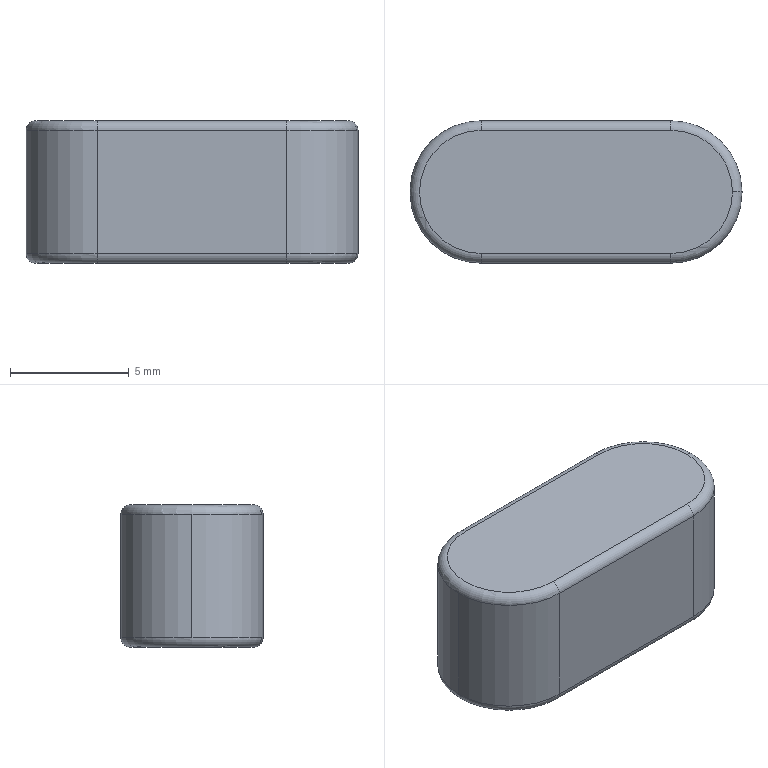Part | SolidWorks | features Extrusion 1, Fillet 1 | 1 solid | 17 faces | box 14 x 6 x 6 mm | volume 455.291 mm3 | cylinder 7 | torus 6 | plane 4 | commonest cylinder face diameters 0.8 x4 6 x3
STEP:
#1=CARTESIAN_POINT('',(6.6,0.,0.));
#2=VERTEX_POINT('',#1);
#3=CARTESIAN_POINT('',(4.,-2.6,0.));
#4=VERTEX_POINT('',#3);
#5=CARTESIAN_POINT('',(4.,0.,0.));
#6=DIRECTION('',(0.,0.,-1.));
#7=DIRECTION('',(1.,0.,0.));
#8=AXIS2_PLACEMENT_3D('',#5,#6,#7);
#9=CIRCLE('',#8,2.6);
#10=EDGE_CURVE('',#2,#4,#9,.T.);
#11=ORIENTED_EDGE('',*,*,#10,.F.);
#12=CARTESIAN_POINT('',(7.,0.,0.4));
#13=VERTEX_POINT('',#12);
#14=CARTESIAN_POINT('',(6.6,0.,0.4));
#15=DIRECTION('',(0.,-1.,0.));
#16=DIRECTION('',(0.,0.,-1.));
#17=AXIS2_PLACEMENT_3D('',#14,#15,#16);
#18=CIRCLE('',#17,0.4);
#19=EDGE_CURVE('',#2,#13,#18,.T.);
#20=ORIENTED_EDGE('',*,*,#19,.T.);
#21=CARTESIAN_POINT('',(4.,-3.,0.4));
#22=VERTEX_POINT('',#21);
#23=CARTESIAN_POINT('',(4.,0.,0.4));
#24=DIRECTION('',(0.,0.,1.));
#25=DIRECTION('',(1.,0.,0.));
#26=AXIS2_PLACEMENT_3D('',#23,#24,#25);
#27=CIRCLE('',#26,3.);
#28=EDGE_CURVE('',#22,#13,#27,.T.);
#29=ORIENTED_EDGE('',*,*,#28,.F.);
#30=CARTESIAN_POINT('',(4.,-2.6,0.4));
#31=DIRECTION('',(1.,0.,0.));
#32=DIRECTION('',(0.,0.,-1.));
#33=AXIS2_PLACEMENT_3D('',#30,#31,#32);
#34=CIRCLE('',#33,0.4);
#35=EDGE_CURVE('',#22,#4,#34,.T.);
#36=ORIENTED_EDGE('',*,*,#35,.T.);
#37=EDGE_LOOP('',(#11,#20,#29,#36));
#38=FACE_OUTER_BOUND('',#37,.T.);
#39=CARTESIAN_POINT('',(4.,0.,0.4));
#40=DIRECTION('',(0.,0.,1.));
#41=DIRECTION('',(1.,0.,0.));
#42=AXIS2_PLACEMENT_3D('',#39,#40,#41);
#43=TOROIDAL_SURFACE('',#42,2.6,0.4);
#44=ADVANCED_FACE('',(#38),#43,.T.);
#45=CARTESIAN_POINT('',(7.,0.,5.6));
#46=VERTEX_POINT('',#45);
#47=CARTESIAN_POINT('',(4.,-3.,5.6));
#48=VERTEX_POINT('',#47);
#49=CARTESIAN_POINT('',(4.,0.,5.6));
#50=DIRECTION('',(0.,0.,-1.));
#51=DIRECTION('',(1.,0.,0.));
#52=AXIS2_PLACEMENT_3D('',#49,#50,#51);
#53=CIRCLE('',#52,3.);
#54=EDGE_CURVE('',#46,#48,#53,.T.);
#55=ORIENTED_EDGE('',*,*,#54,.F.);
#56=CARTESIAN_POINT('',(6.6,0.,6.));
#57=VERTEX_POINT('',#56);
#58=CARTESIAN_POINT('',(6.6,0.,5.6));
#59=DIRECTION('',(0.,-1.,0.));
#60=DIRECTION('',(0.,0.,-1.));
#61=AXIS2_PLACEMENT_3D('',#58,#59,#60);
#62=CIRCLE('',#61,0.4);
#63=EDGE_CURVE('',#46,#57,#62,.T.);
#64=ORIENTED_EDGE('',*,*,#63,.T.);
#65=CARTESIAN_POINT('',(4.,-2.6,6.));
#66=VERTEX_POINT('',#65);
#67=CARTESIAN_POINT('',(4.,0.,6.));
#68=DIRECTION('',(0.,0.,1.));
#69=DIRECTION('',(1.,0.,0.));
#70=AXIS2_PLACEMENT_3D('',#67,#68,#69);
#71=CIRCLE('',#70,2.6);
#72=EDGE_CURVE('',#66,#57,#71,.T.);
#73=ORIENTED_EDGE('',*,*,#72,.F.);
#74=CARTESIAN_POINT('',(4.,-2.6,5.6));
#75=DIRECTION('',(1.,0.,0.));
#76=DIRECTION('',(0.,0.,-1.));
#77=AXIS2_PLACEMENT_3D('',#74,#75,#76);
#78=CIRCLE('',#77,0.4);
#79=EDGE_CURVE('',#66,#48,#78,.T.);
#80=ORIENTED_EDGE('',*,*,#79,.T.);
#81=EDGE_LOOP('',(#55,#64,#73,#80));
#82=FACE_OUTER_BOUND('',#81,.T.);
#83=CARTESIAN_POINT('',(4.,0.,5.6));
#84=DIRECTION('',(0.,0.,1.));
#85=DIRECTION('',(1.,0.,0.));
#86=AXIS2_PLACEMENT_3D('',#83,#84,#85);
#87=TOROIDAL_SURFACE('',#86,2.6,0.4);
#88=ADVANCED_FACE('',(#82),#87,.T.);
#89=CARTESIAN_POINT('',(-4.,-3.,5.6));
#90=VERTEX_POINT('',#89);
#91=CARTESIAN_POINT('',(-7.,0.,5.6));
#92=VERTEX_POINT('',#91);
#93=CARTESIAN_POINT('',(-4.,0.,5.6));
#94=DIRECTION('',(0.,0.,-1.));
#95=DIRECTION('',(1.,0.,0.));
#96=AXIS2_PLACEMENT_3D('',#93,#94,#95);
#97=CIRCLE('',#96,3.);
#98=EDGE_CURVE('',#90,#92,#97,.T.);
#99=ORIENTED_EDGE('',*,*,#98,.T.);
#100=CARTESIAN_POINT('',(-7.,0.,0.4));
#101=VERTEX_POINT('',#100);
#102=CARTESIAN_POINT('',(-7.,0.,6.));
#103=DIRECTION('',(0.,0.,-1.));
#104=VECTOR('',#103,1000.);
#105=LINE('',#102,#104);
#106=EDGE_CURVE('',#92,#101,#105,.T.);
#107=ORIENTED_EDGE('',*,*,#106,.T.);
#108=CARTESIAN_POINT('',(-4.,-3.,0.4));
#109=VERTEX_POINT('',#108);
#110=CARTESIAN_POINT('',(-4.,0.,0.4));
#111=DIRECTION('',(0.,0.,1.));
#112=DIRECTION('',(1.,0.,0.));
#113=AXIS2_PLACEMENT_3D('',#110,#111,#112);
#114=CIRCLE('',#113,3.);
#115=EDGE_CURVE('',#101,#109,#114,.T.);
#116=ORIENTED_EDGE('',*,*,#115,.T.);
#117=CARTESIAN_POINT('',(-4.,-3.,6.));
#118=DIRECTION('',(0.,0.,-1.));
#119=VECTOR('',#118,1000.);
#120=LINE('',#117,#119);
#121=EDGE_CURVE('',#90,#109,#120,.T.);
#122=ORIENTED_EDGE('',*,*,#121,.F.);
#123=EDGE_LOOP('',(#99,#107,#116,#122));
#124=FACE_OUTER_BOUND('',#123,.T.);
#125=CARTESIAN_POINT('',(-4.,0.,6.));
#126=DIRECTION('',(0.,0.,-1.));
#127=DIRECTION('',(-1.,0.,0.));
#128=AXIS2_PLACEMENT_3D('',#125,#126,#127);
#129=CYLINDRICAL_SURFACE('',#128,3.);
#130=ADVANCED_FACE('',(#124),#129,.T.);
#131=ORIENTED_EDGE('',*,*,#106,.F.);
#132=CARTESIAN_POINT('',(-4.,3.,5.6));
#133=VERTEX_POINT('',#132);
#134=CARTESIAN_POINT('',(-4.,0.,5.6));
#135=DIRECTION('',(0.,0.,-1.));
#136=DIRECTION('',(1.,0.,0.));
#137=AXIS2_PLACEMENT_3D('',#134,#135,#136);
#138=CIRCLE('',#137,3.);
#139=EDGE_CURVE('',#92,#133,#138,.T.);
#140=ORIENTED_EDGE('',*,*,#139,.T.);
#141=CARTESIAN_POINT('',(-4.,3.,0.4));
#142=VERTEX_POINT('',#141);
#143=CARTESIAN_POINT('',(-4.,3.,6.));
#144=DIRECTION('',(0.,0.,-1.));
#145=VECTOR('',#144,1000.);
#146=LINE('',#143,#145);
#147=EDGE_CURVE('',#133,#142,#146,.T.);
#148=ORIENTED_EDGE('',*,*,#147,.T.);
#149=CARTESIAN_POINT('',(-4.,0.,0.4));
#150=DIRECTION('',(0.,0.,1.));
#151=DIRECTION('',(1.,0.,0.));
#152=AXIS2_PLACEMENT_3D('',#149,#150,#151);
#153=CIRCLE('',#152,3.);
#154=EDGE_CURVE('',#142,#101,#153,.T.);
#155=ORIENTED_EDGE('',*,*,#154,.T.);
#156=EDGE_LOOP('',(#131,#140,#148,#155));
#157=FACE_OUTER_BOUND('',#156,.T.);
#158=CARTESIAN_POINT('',(-4.,0.,6.));
#159=DIRECTION('',(0.,0.,-1.));
#160=DIRECTION('',(-1.,0.,0.));
#161=AXIS2_PLACEMENT_3D('',#158,#159,#160);
#162=CYLINDRICAL_SURFACE('',#161,3.);
#163=ADVANCED_FACE('',(#157),#162,.T.);
#164=CARTESIAN_POINT('',(4.,-3.,6.));
#165=DIRECTION('',(0.,0.,-1.));
#166=VECTOR('',#165,1000.);
#167=LINE('',#164,#166);
#168=EDGE_CURVE('',#48,#22,#167,.T.);
#169=ORIENTED_EDGE('',*,*,#168,.F.);
#170=CARTESIAN_POINT('',(-4.,-3.,5.6));
#171=DIRECTION('',(-1.,0.,0.));
#172=VECTOR('',#171,1000.);
#173=LINE('',#170,#172);
#174=EDGE_CURVE('',#48,#90,#173,.T.);
#175=ORIENTED_EDGE('',*,*,#174,.T.);
#176=ORIENTED_EDGE('',*,*,#121,.T.);
#177=CARTESIAN_POINT('',(-4.,-3.,0.4));
#178=DIRECTION('',(1.,0.,0.));
#179=VECTOR('',#178,1000.);
#180=LINE('',#177,#179);
#181=EDGE_CURVE('',#109,#22,#180,.T.);
#182=ORIENTED_EDGE('',*,*,#181,.T.);
#183=EDGE_LOOP('',(#169,#175,#176,#182));
#184=FACE_OUTER_BOUND('',#183,.T.);
#185=CARTESIAN_POINT('',(-4.,-3.,6.));
#186=DIRECTION('',(0.,1.,0.));
#187=DIRECTION('',(-1.,0.,0.));
#188=AXIS2_PLACEMENT_3D('',#185,#186,#187);
#189=PLANE('',#188);
#190=ADVANCED_FACE('',(#184),#189,.F.);
#191=CARTESIAN_POINT('',(4.,3.,5.6));
#192=VERTEX_POINT('',#191);
#193=CARTESIAN_POINT('',(4.,3.,0.4));
#194=VERTEX_POINT('',#193);
#195=CARTESIAN_POINT('',(4.,3.,6.));
#196=DIRECTION('',(0.,0.,-1.));
#197=VECTOR('',#196,1000.);
#198=LINE('',#195,#197);
#199=EDGE_CURVE('',#192,#194,#198,.T.);
#200=ORIENTED_EDGE('',*,*,#199,.F.);
#201=CARTESIAN_POINT('',(4.,0.,5.6));
#202=DIRECTION('',(0.,0.,-1.));
#203=DIRECTION('',(1.,0.,0.));
#204=AXIS2_PLACEMENT_3D('',#201,#202,#203);
#205=CIRCLE('',#204,3.);
#206=EDGE_CURVE('',#192,#46,#205,.T.);
#207=ORIENTED_EDGE('',*,*,#206,.T.);
#208=ORIENTED_EDGE('',*,*,#54,.T.);
#209=ORIENTED_EDGE('',*,*,#168,.T.);
#210=ORIENTED_EDGE('',*,*,#28,.T.);
#211=CARTESIAN_POINT('',(4.,0.,0.4));
#212=DIRECTION('',(0.,0.,1.));
#213=DIRECTION('',(1.,0.,0.));
#214=AXIS2_PLACEMENT_3D('',#211,#212,#213);
#215=CIRCLE('',#214,3.);
#216=EDGE_CURVE('',#13,#194,#215,.T.);
#217=ORIENTED_EDGE('',*,*,#216,.T.);
#218=EDGE_LOOP('',(#200,#207,#208,#209,#210,#217));
#219=FACE_OUTER_BOUND('',#218,.T.);
#220=CARTESIAN_POINT('',(4.,0.,6.));
#221=DIRECTION('',(0.,0.,-1.));
#222=DIRECTION('',(-1.,0.,0.));
#223=AXIS2_PLACEMENT_3D('',#220,#221,#222);
#224=CYLINDRICAL_SURFACE('',#223,3.);
#225=ADVANCED_FACE('',(#219),#224,.T.);
#226=ORIENTED_EDGE('',*,*,#147,.F.);
#227=CARTESIAN_POINT('',(4.,3.,5.6));
#228=DIRECTION('',(1.,0.,0.));
#229=VECTOR('',#228,1000.);
#230=LINE('',#227,#229);
#231=EDGE_CURVE('',#133,#192,#230,.T.);
#232=ORIENTED_EDGE('',*,*,#231,.T.);
#233=ORIENTED_EDGE('',*,*,#199,.T.);
#234=CARTESIAN_POINT('',(-4.,3.,0.4));
#235=DIRECTION('',(-1.,0.,0.));
#236=VECTOR('',#235,1000.);
#237=LINE('',#234,#236);
#238=EDGE_CURVE('',#194,#142,#237,.T.);
#239=ORIENTED_EDGE('',*,*,#238,.T.);
#240=EDGE_LOOP('',(#226,#232,#233,#239));
#241=FACE_OUTER_BOUND('',#240,.T.);
#242=CARTESIAN_POINT('',(-4.,3.,6.));
#243=DIRECTION('',(0.,-1.,0.));
#244=DIRECTION('',(1.,0.,0.));
#245=AXIS2_PLACEMENT_3D('',#242,#243,#244);
#246=PLANE('',#245);
#247=ADVANCED_FACE('',(#241),#246,.F.);
#248=CARTESIAN_POINT('',(-4.,-2.6,6.));
#249=VERTEX_POINT('',#248);
#250=CARTESIAN_POINT('',(4.,-2.6,6.));
#251=DIRECTION('',(1.,0.,0.));
#252=VECTOR('',#251,1000.);
#253=LINE('',#250,#252);
#254=EDGE_CURVE('',#249,#66,#253,.T.);
#255=ORIENTED_EDGE('',*,*,#254,.T.);
#256=ORIENTED_EDGE('',*,*,#72,.T.);
#257=CARTESIAN_POINT('',(4.,2.6,6.));
#258=VERTEX_POINT('',#257);
#259=CARTESIAN_POINT('',(4.,0.,6.));
#260=DIRECTION('',(0.,0.,1.));
#261=DIRECTION('',(1.,0.,0.));
#262=AXIS2_PLACEMENT_3D('',#259,#260,#261);
#263=CIRCLE('',#262,2.6);
#264=EDGE_CURVE('',#57,#258,#263,.T.);
#265=ORIENTED_EDGE('',*,*,#264,.T.);
#266=CARTESIAN_POINT('',(-4.,2.6,6.));
#267=VERTEX_POINT('',#266);
#268=CARTESIAN_POINT('',(-4.,2.6,6.));
#269=DIRECTION('',(-1.,0.,0.));
#270=VECTOR('',#269,1000.);
#271=LINE('',#268,#270);
#272=EDGE_CURVE('',#258,#267,#271,.T.);
#273=ORIENTED_EDGE('',*,*,#272,.T.);
#274=CARTESIAN_POINT('',(-4.,0.,6.));
#275=DIRECTION('',(0.,0.,1.));
#276=DIRECTION('',(1.,0.,0.));
#277=AXIS2_PLACEMENT_3D('',#274,#275,#276);
#278=CIRCLE('',#277,2.6);
#279=EDGE_CURVE('',#267,#249,#278,.T.);
#280=ORIENTED_EDGE('',*,*,#279,.T.);
#281=EDGE_LOOP('',(#255,#256,#265,#273,#280));
#282=FACE_OUTER_BOUND('',#281,.T.);
#283=CARTESIAN_POINT('',(-4.,0.,6.));
#284=DIRECTION('',(0.,0.,1.));
#285=DIRECTION('',(1.,0.,0.));
#286=AXIS2_PLACEMENT_3D('',#283,#284,#285);
#287=PLANE('',#286);
#288=ADVANCED_FACE('',(#282),#287,.T.);
#289=CARTESIAN_POINT('',(-4.,2.6,0.));
#290=VERTEX_POINT('',#289);
#291=CARTESIAN_POINT('',(4.,2.6,0.));
#292=VERTEX_POINT('',#291);
#293=CARTESIAN_POINT('',(-4.,2.6,0.));
#294=DIRECTION('',(1.,0.,0.));
#295=VECTOR('',#294,1000.);
#296=LINE('',#293,#295);
#297=EDGE_CURVE('',#290,#292,#296,.T.);
#298=ORIENTED_EDGE('',*,*,#297,.T.);
#299=CARTESIAN_POINT('',(4.,0.,0.));
#300=DIRECTION('',(0.,0.,-1.));
#301=DIRECTION('',(1.,0.,0.));
#302=AXIS2_PLACEMENT_3D('',#299,#300,#301);
#303=CIRCLE('',#302,2.6);
#304=EDGE_CURVE('',#292,#2,#303,.T.);
#305=ORIENTED_EDGE('',*,*,#304,.T.);
#306=ORIENTED_EDGE('',*,*,#10,.T.);
#307=CARTESIAN_POINT('',(-4.,-2.6,0.));
#308=VERTEX_POINT('',#307);
#309=CARTESIAN_POINT('',(-4.,-2.6,0.));
#310=DIRECTION('',(-1.,0.,0.));
#311=VECTOR('',#310,1000.);
#312=LINE('',#309,#311);
#313=EDGE_CURVE('',#4,#308,#312,.T.);
#314=ORIENTED_EDGE('',*,*,#313,.T.);
#315=CARTESIAN_POINT('',(-4.,0.,0.));
#316=DIRECTION('',(0.,0.,-1.));
#317=DIRECTION('',(1.,0.,0.));
#318=AXIS2_PLACEMENT_3D('',#315,#316,#317);
#319=CIRCLE('',#318,2.6);
#320=EDGE_CURVE('',#308,#290,#319,.T.);
#321=ORIENTED_EDGE('',*,*,#320,.T.);
#322=EDGE_LOOP('',(#298,#305,#306,#314,#321));
#323=FACE_OUTER_BOUND('',#322,.T.);
#324=CARTESIAN_POINT('',(-4.,0.,0.));
#325=DIRECTION('',(0.,0.,1.));
#326=DIRECTION('',(1.,0.,0.));
#327=AXIS2_PLACEMENT_3D('',#324,#325,#326);
#328=PLANE('',#327);
#329=ADVANCED_FACE('',(#323),#328,.F.);
#330=CARTESIAN_POINT('',(-4.,2.6,5.6));
#331=DIRECTION('',(1.,0.,0.));
#332=DIRECTION('',(0.,0.,-1.));
#333=AXIS2_PLACEMENT_3D('',#330,#331,#332);
#334=CIRCLE('',#333,0.4);
#335=EDGE_CURVE('',#133,#267,#334,.T.);
#336=ORIENTED_EDGE('',*,*,#335,.F.);
#337=ORIENTED_EDGE('',*,*,#139,.F.);
#338=ORIENTED_EDGE('',*,*,#98,.F.);
#339=CARTESIAN_POINT('',(-4.,-2.6,5.6));
#340=DIRECTION('',(1.,0.,0.));
#341=DIRECTION('',(0.,0.,-1.));
#342=AXIS2_PLACEMENT_3D('',#339,#340,#341);
#343=CIRCLE('',#342,0.4);
#344=EDGE_CURVE('',#249,#90,#343,.T.);
#345=ORIENTED_EDGE('',*,*,#344,.F.);
#346=ORIENTED_EDGE('',*,*,#279,.F.);
#347=EDGE_LOOP('',(#336,#337,#338,#345,#346));
#348=FACE_OUTER_BOUND('',#347,.T.);
#349=CARTESIAN_POINT('',(-4.,0.,5.6));
#350=DIRECTION('',(0.,0.,1.));
#351=DIRECTION('',(1.,0.,0.));
#352=AXIS2_PLACEMENT_3D('',#349,#350,#351);
#353=TOROIDAL_SURFACE('',#352,2.6,0.4);
#354=ADVANCED_FACE('',(#348),#353,.T.);
#355=ORIENTED_EDGE('',*,*,#344,.T.);
#356=ORIENTED_EDGE('',*,*,#174,.F.);
#357=ORIENTED_EDGE('',*,*,#79,.F.);
#358=ORIENTED_EDGE('',*,*,#254,.F.);
#359=EDGE_LOOP('',(#355,#356,#357,#358));
#360=FACE_OUTER_BOUND('',#359,.T.);
#361=CARTESIAN_POINT('',(-4.,-2.6,5.6));
#362=DIRECTION('',(-1.,0.,0.));
#363=DIRECTION('',(0.,-1.,0.));
#364=AXIS2_PLACEMENT_3D('',#361,#362,#363);
#365=CYLINDRICAL_SURFACE('',#364,0.4);
#366=ADVANCED_FACE('',(#360),#365,.T.);
#367=ORIENTED_EDGE('',*,*,#335,.T.);
#368=ORIENTED_EDGE('',*,*,#272,.F.);
#369=CARTESIAN_POINT('',(4.,2.6,5.6));
#370=DIRECTION('',(1.,0.,0.));
#371=DIRECTION('',(0.,0.,-1.));
#372=AXIS2_PLACEMENT_3D('',#369,#370,#371);
#373=CIRCLE('',#372,0.4);
#374=EDGE_CURVE('',#192,#258,#373,.T.);
#375=ORIENTED_EDGE('',*,*,#374,.F.);
#376=ORIENTED_EDGE('',*,*,#231,.F.);
#377=EDGE_LOOP('',(#367,#368,#375,#376));
#378=FACE_OUTER_BOUND('',#377,.T.);
#379=CARTESIAN_POINT('',(-4.,2.6,5.6));
#380=DIRECTION('',(1.,0.,0.));
#381=DIRECTION('',(0.,1.,0.));
#382=AXIS2_PLACEMENT_3D('',#379,#380,#381);
#383=CYLINDRICAL_SURFACE('',#382,0.4);
#384=ADVANCED_FACE('',(#378),#383,.T.);
#385=ORIENTED_EDGE('',*,*,#63,.F.);
#386=ORIENTED_EDGE('',*,*,#206,.F.);
#387=ORIENTED_EDGE('',*,*,#374,.T.);
#388=ORIENTED_EDGE('',*,*,#264,.F.);
#389=EDGE_LOOP('',(#385,#386,#387,#388));
#390=FACE_OUTER_BOUND('',#389,.T.);
#391=CARTESIAN_POINT('',(4.,0.,5.6));
#392=DIRECTION('',(0.,0.,1.));
#393=DIRECTION('',(1.,0.,0.));
#394=AXIS2_PLACEMENT_3D('',#391,#392,#393);
#395=TOROIDAL_SURFACE('',#394,2.6,0.4);
#396=ADVANCED_FACE('',(#390),#395,.T.);
#397=CARTESIAN_POINT('',(-4.,2.6,0.4));
#398=DIRECTION('',(1.,0.,0.));
#399=DIRECTION('',(0.,0.,-1.));
#400=AXIS2_PLACEMENT_3D('',#397,#398,#399);
#401=CIRCLE('',#400,0.4);
#402=EDGE_CURVE('',#290,#142,#401,.T.);
#403=ORIENTED_EDGE('',*,*,#402,.F.);
#404=ORIENTED_EDGE('',*,*,#320,.F.);
#405=CARTESIAN_POINT('',(-4.,-2.6,0.4));
#406=DIRECTION('',(1.,0.,0.));
#407=DIRECTION('',(0.,0.,-1.));
#408=AXIS2_PLACEMENT_3D('',#405,#406,#407);
#409=CIRCLE('',#408,0.4);
#410=EDGE_CURVE('',#109,#308,#409,.T.);
#411=ORIENTED_EDGE('',*,*,#410,.F.);
#412=ORIENTED_EDGE('',*,*,#115,.F.);
#413=ORIENTED_EDGE('',*,*,#154,.F.);
#414=EDGE_LOOP('',(#403,#404,#411,#412,#413));
#415=FACE_OUTER_BOUND('',#414,.T.);
#416=CARTESIAN_POINT('',(-4.,0.,0.4));
#417=DIRECTION('',(0.,0.,1.));
#418=DIRECTION('',(1.,0.,0.));
#419=AXIS2_PLACEMENT_3D('',#416,#417,#418);
#420=TOROIDAL_SURFACE('',#419,2.6,0.4);
#421=ADVANCED_FACE('',(#415),#420,.T.);
#422=ORIENTED_EDGE('',*,*,#410,.T.);
#423=ORIENTED_EDGE('',*,*,#313,.F.);
#424=ORIENTED_EDGE('',*,*,#35,.F.);
#425=ORIENTED_EDGE('',*,*,#181,.F.);
#426=EDGE_LOOP('',(#422,#423,#424,#425));
#427=FACE_OUTER_BOUND('',#426,.T.);
#428=CARTESIAN_POINT('',(-4.,-2.6,0.4));
#429=DIRECTION('',(1.,0.,0.));
#430=DIRECTION('',(0.,1.,0.));
#431=AXIS2_PLACEMENT_3D('',#428,#429,#430);
#432=CYLINDRICAL_SURFACE('',#431,0.4);
#433=ADVANCED_FACE('',(#427),#432,.T.);
#434=ORIENTED_EDGE('',*,*,#402,.T.);
#435=ORIENTED_EDGE('',*,*,#238,.F.);
#436=CARTESIAN_POINT('',(4.,2.6,0.4));
#437=DIRECTION('',(1.,0.,0.));
#438=DIRECTION('',(0.,0.,-1.));
#439=AXIS2_PLACEMENT_3D('',#436,#437,#438);
#440=CIRCLE('',#439,0.4);
#441=EDGE_CURVE('',#292,#194,#440,.T.);
#442=ORIENTED_EDGE('',*,*,#441,.F.);
#443=ORIENTED_EDGE('',*,*,#297,.F.);
#444=EDGE_LOOP('',(#434,#435,#442,#443));
#445=FACE_OUTER_BOUND('',#444,.T.);
#446=CARTESIAN_POINT('',(-4.,2.6,0.4));
#447=DIRECTION('',(-1.,0.,0.));
#448=DIRECTION('',(0.,-1.,0.));
#449=AXIS2_PLACEMENT_3D('',#446,#447,#448);
#450=CYLINDRICAL_SURFACE('',#449,0.4);
#451=ADVANCED_FACE('',(#445),#450,.T.);
#452=ORIENTED_EDGE('',*,*,#19,.F.);
#453=ORIENTED_EDGE('',*,*,#304,.F.);
#454=ORIENTED_EDGE('',*,*,#441,.T.);
#455=ORIENTED_EDGE('',*,*,#216,.F.);
#456=EDGE_LOOP('',(#452,#453,#454,#455));
#457=FACE_OUTER_BOUND('',#456,.T.);
#458=CARTESIAN_POINT('',(4.,0.,0.4));
#459=DIRECTION('',(0.,0.,1.));
#460=DIRECTION('',(1.,0.,0.));
#461=AXIS2_PLACEMENT_3D('',#458,#459,#460);
#462=TOROIDAL_SURFACE('',#461,2.6,0.4);
#463=ADVANCED_FACE('',(#457),#462,.T.);
#464=CLOSED_SHELL('',(#44,#88,#130,#163,#190,#225,#247,#288,#329,#354,#366,#384,#396,#421,#433,#451,#463));
#465=MANIFOLD_SOLID_BREP('',#464);
#466=CARTESIAN_POINT('',(0.,0.,0.));
#467=DIRECTION('',(0.,0.,1.));
#468=DIRECTION('',(1.,0.,0.));
#469=AXIS2_PLACEMENT_3D('',#466,#467,#468);
#470=(LENGTH_UNIT()NAMED_UNIT(*)SI_UNIT(.MILLI.,.METRE.));
#471=UNCERTAINTY_MEASURE_WITH_UNIT(LENGTH_MEASURE(0.00001),#470,'','');
#472=(NAMED_UNIT(*)PLANE_ANGLE_UNIT()SI_UNIT($,.RADIAN.));
#473=(NAMED_UNIT(*)SI_UNIT($,.STERADIAN.)SOLID_ANGLE_UNIT());
#474=(GEOMETRIC_REPRESENTATION_CONTEXT(3)GLOBAL_UNCERTAINTY_ASSIGNED_CONTEXT((#471))GLOBAL_UNIT_ASSIGNED_CONTEXT((#470,#472,#473))REPRESENTATION_CONTEXT('',''));
#475=ADVANCED_BREP_SHAPE_REPRESENTATION('',(#465,#469),#474);